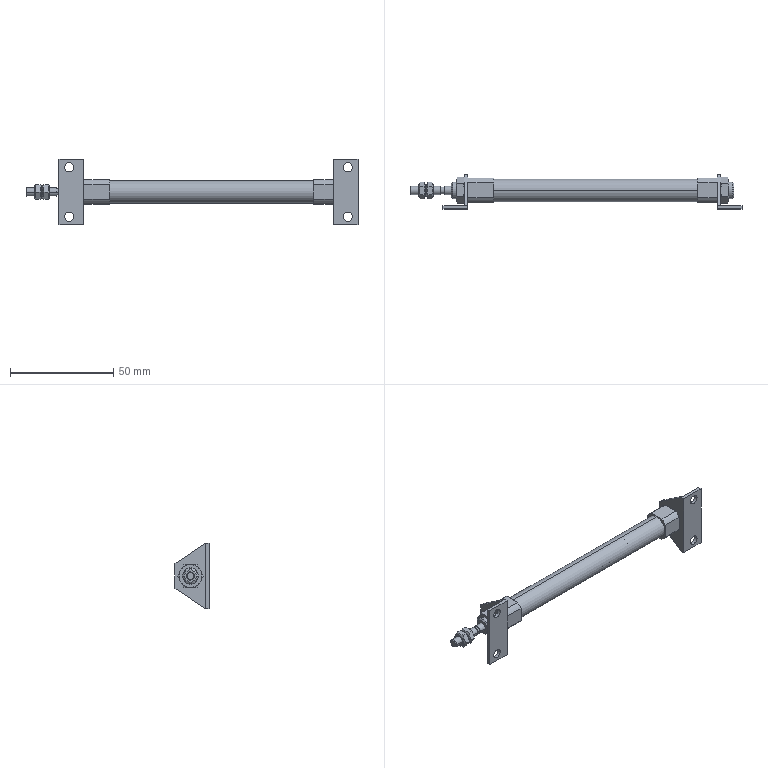Part | STEP file | CDJ2M10-75Z-B_0_0_0_^Take-up clamp assembly | 8 solids | 193 faces | box 161 x 16.5 x 32 mm | volume 11059 mm3 | plane 73 | cone 70 | cylinder 50 | commonest cylinder face diameters 4.5 x8 8 x8 14 x8 4 x6 3.242 x4 4.134 x4